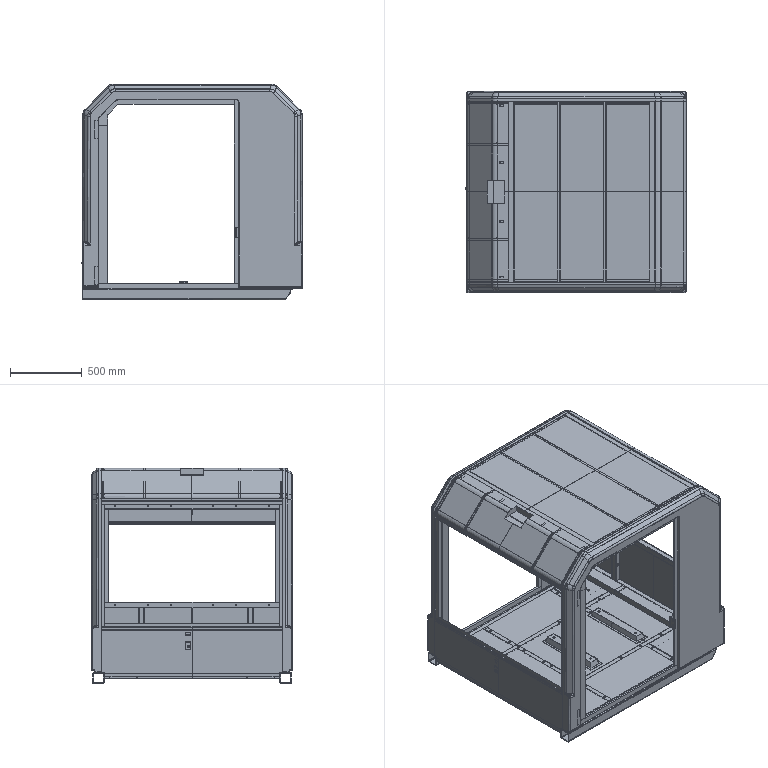Part | NX | features BREP 44 | 107 solids | 3775 faces | volume 35333668 mm3 | plane 1757 | cylinder 1520 | spline 287 | cone 93 | torus 91 | sphere 27 | commonest cylinder face diameters 6 x306 10 x197 15 x192 8 x149 6.5 x136 4 x106